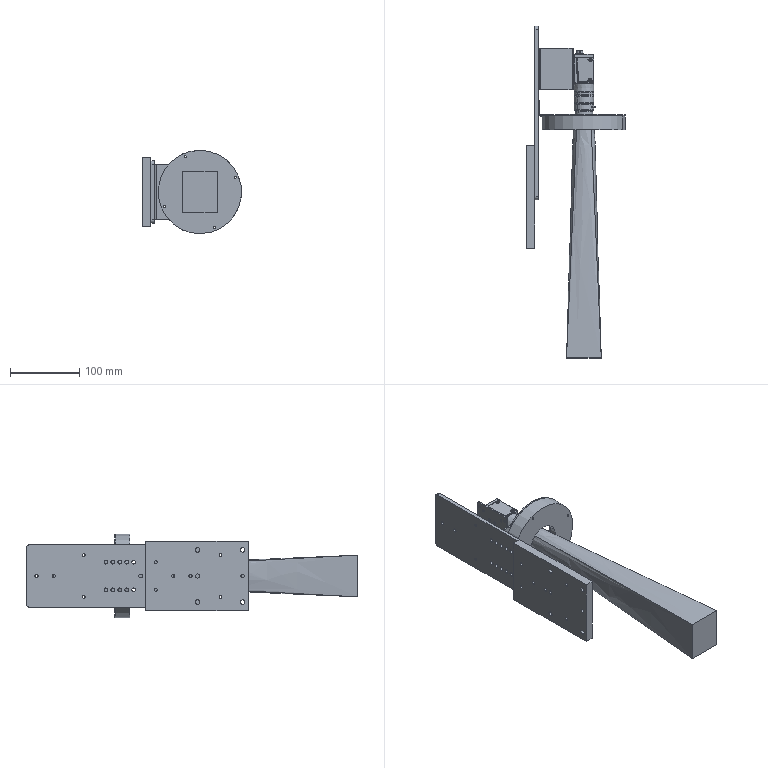Part | SolidWorks | features ReferencePattern 6, InContextFeatHolder 2, CompositeCurve 1, LocalLPattern 1 | 10 solids | 1452 faces | box 142.5 x 477.965 x 120 mm | volume 1151142 mm3 | plane 597 | cylinder 402 | spline 255 | cone 196 | torus 2 | commonest cylinder face diameters 5.5 x60 3 x26 4 x24 2 x22 0.8 x16 0.814 x16